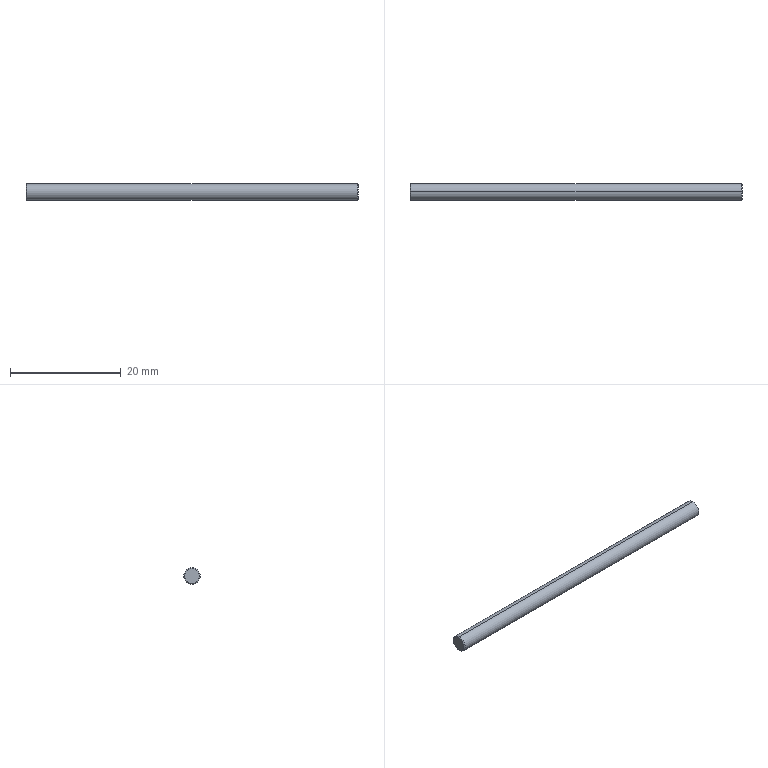Part | SolidWorks | features Chamfer 1, Extrusion 1 | 1 solid | 8 faces | box 60 x 3 x 3 mm | volume 423.91 mm3 | cone 4 | cylinder 2 | plane 2 | commonest cylinder face diameters 3 x2
STEP:
#1=CARTESIAN_POINT('',(30.,0.,-1.35));
#2=VERTEX_POINT('',#1);
#3=CARTESIAN_POINT('',(30.,0.,1.35));
#4=VERTEX_POINT('',#3);
#5=CARTESIAN_POINT('',(30.,0.,0.));
#6=DIRECTION('',(1.,0.,0.));
#7=DIRECTION('',(0.,0.,-1.));
#8=AXIS2_PLACEMENT_3D('',#5,#6,#7);
#9=CIRCLE('',#8,1.35);
#10=EDGE_CURVE('',#2,#4,#9,.T.);
#11=ORIENTED_EDGE('',*,*,#10,.F.);
#12=CARTESIAN_POINT('',(29.85,0.,-1.5));
#13=VERTEX_POINT('',#12);
#14=CARTESIAN_POINT('',(30.,0.,-1.35));
#15=DIRECTION('',(-0.7071,0.,-0.7071));
#16=VECTOR('',#15,1000.);
#17=LINE('',#14,#16);
#18=EDGE_CURVE('',#2,#13,#17,.T.);
#19=ORIENTED_EDGE('',*,*,#18,.T.);
#20=CARTESIAN_POINT('',(29.85,0.,1.5));
#21=VERTEX_POINT('',#20);
#22=CARTESIAN_POINT('',(29.85,0.,0.));
#23=DIRECTION('',(-1.,0.,0.));
#24=DIRECTION('',(0.,0.,-1.));
#25=AXIS2_PLACEMENT_3D('',#22,#23,#24);
#26=CIRCLE('',#25,1.5);
#27=EDGE_CURVE('',#21,#13,#26,.T.);
#28=ORIENTED_EDGE('',*,*,#27,.F.);
#29=CARTESIAN_POINT('',(30.,0.,1.35));
#30=DIRECTION('',(-0.7071,0.,0.7071));
#31=VECTOR('',#30,1000.);
#32=LINE('',#29,#31);
#33=EDGE_CURVE('',#4,#21,#32,.T.);
#34=ORIENTED_EDGE('',*,*,#33,.F.);
#35=EDGE_LOOP('',(#11,#19,#28,#34));
#36=FACE_OUTER_BOUND('',#35,.T.);
#37=CARTESIAN_POINT('',(30.,0.,0.));
#38=DIRECTION('',(-1.,0.,0.));
#39=DIRECTION('',(0.,0.,1.));
#40=AXIS2_PLACEMENT_3D('',#37,#38,#39);
#41=CONICAL_SURFACE('',#40,1.35,0.7854);
#42=ADVANCED_FACE('',(#36),#41,.T.);
#43=CARTESIAN_POINT('',(-30.,0.,1.35));
#44=VERTEX_POINT('',#43);
#45=CARTESIAN_POINT('',(-30.,0.,-1.35));
#46=VERTEX_POINT('',#45);
#47=CARTESIAN_POINT('',(-30.,0.,0.));
#48=DIRECTION('',(-1.,0.,0.));
#49=DIRECTION('',(0.,0.,-1.));
#50=AXIS2_PLACEMENT_3D('',#47,#48,#49);
#51=CIRCLE('',#50,1.35);
#52=EDGE_CURVE('',#44,#46,#51,.T.);
#53=ORIENTED_EDGE('',*,*,#52,.F.);
#54=CARTESIAN_POINT('',(-29.85,0.,1.5));
#55=VERTEX_POINT('',#54);
#56=CARTESIAN_POINT('',(-29.85,0.,1.5));
#57=DIRECTION('',(0.7071,0.,0.7071));
#58=VECTOR('',#57,1000.);
#59=LINE('',#56,#58);
#60=EDGE_CURVE('',#44,#55,#59,.T.);
#61=ORIENTED_EDGE('',*,*,#60,.T.);
#62=CARTESIAN_POINT('',(-29.85,0.,-1.5));
#63=VERTEX_POINT('',#62);
#64=CARTESIAN_POINT('',(-29.85,0.,0.));
#65=DIRECTION('',(1.,0.,0.));
#66=DIRECTION('',(0.,0.,-1.));
#67=AXIS2_PLACEMENT_3D('',#64,#65,#66);
#68=CIRCLE('',#67,1.5);
#69=EDGE_CURVE('',#63,#55,#68,.T.);
#70=ORIENTED_EDGE('',*,*,#69,.F.);
#71=CARTESIAN_POINT('',(-29.85,0.,-1.5));
#72=DIRECTION('',(0.7071,0.,-0.7071));
#73=VECTOR('',#72,1000.);
#74=LINE('',#71,#73);
#75=EDGE_CURVE('',#46,#63,#74,.T.);
#76=ORIENTED_EDGE('',*,*,#75,.F.);
#77=EDGE_LOOP('',(#53,#61,#70,#76));
#78=FACE_OUTER_BOUND('',#77,.T.);
#79=CARTESIAN_POINT('',(-29.85,0.,0.));
#80=DIRECTION('',(1.,0.,0.));
#81=DIRECTION('',(0.,0.,-1.));
#82=AXIS2_PLACEMENT_3D('',#79,#80,#81);
#83=CONICAL_SURFACE('',#82,1.5,0.7854);
#84=ADVANCED_FACE('',(#78),#83,.T.);
#85=ORIENTED_EDGE('',*,*,#27,.T.);
#86=CARTESIAN_POINT('',(30.,0.,-1.5));
#87=DIRECTION('',(-1.,0.,0.));
#88=VECTOR('',#87,1000.);
#89=LINE('',#86,#88);
#90=EDGE_CURVE('',#13,#63,#89,.T.);
#91=ORIENTED_EDGE('',*,*,#90,.T.);
#92=ORIENTED_EDGE('',*,*,#69,.T.);
#93=CARTESIAN_POINT('',(30.,0.,1.5));
#94=DIRECTION('',(-1.,0.,0.));
#95=VECTOR('',#94,1000.);
#96=LINE('',#93,#95);
#97=EDGE_CURVE('',#21,#55,#96,.T.);
#98=ORIENTED_EDGE('',*,*,#97,.F.);
#99=EDGE_LOOP('',(#85,#91,#92,#98));
#100=FACE_OUTER_BOUND('',#99,.T.);
#101=CARTESIAN_POINT('',(30.,0.,0.));
#102=DIRECTION('',(-1.,0.,0.));
#103=DIRECTION('',(0.,0.,1.));
#104=AXIS2_PLACEMENT_3D('',#101,#102,#103);
#105=CYLINDRICAL_SURFACE('',#104,1.5);
#106=ADVANCED_FACE('',(#100),#105,.T.);
#107=ORIENTED_EDGE('',*,*,#90,.F.);
#108=CARTESIAN_POINT('',(29.85,0.,0.));
#109=DIRECTION('',(-1.,0.,0.));
#110=DIRECTION('',(0.,0.,-1.));
#111=AXIS2_PLACEMENT_3D('',#108,#109,#110);
#112=CIRCLE('',#111,1.5);
#113=EDGE_CURVE('',#13,#21,#112,.T.);
#114=ORIENTED_EDGE('',*,*,#113,.T.);
#115=ORIENTED_EDGE('',*,*,#97,.T.);
#116=CARTESIAN_POINT('',(-29.85,0.,0.));
#117=DIRECTION('',(1.,0.,0.));
#118=DIRECTION('',(0.,0.,-1.));
#119=AXIS2_PLACEMENT_3D('',#116,#117,#118);
#120=CIRCLE('',#119,1.5);
#121=EDGE_CURVE('',#55,#63,#120,.T.);
#122=ORIENTED_EDGE('',*,*,#121,.T.);
#123=EDGE_LOOP('',(#107,#114,#115,#122));
#124=FACE_OUTER_BOUND('',#123,.T.);
#125=CARTESIAN_POINT('',(30.,0.,0.));
#126=DIRECTION('',(-1.,0.,0.));
#127=DIRECTION('',(0.,0.,1.));
#128=AXIS2_PLACEMENT_3D('',#125,#126,#127);
#129=CYLINDRICAL_SURFACE('',#128,1.5);
#130=ADVANCED_FACE('',(#124),#129,.T.);
#131=CARTESIAN_POINT('',(30.,0.,0.));
#132=DIRECTION('',(1.,0.,0.));
#133=DIRECTION('',(0.,0.,-1.));
#134=AXIS2_PLACEMENT_3D('',#131,#132,#133);
#135=CIRCLE('',#134,1.35);
#136=EDGE_CURVE('',#4,#2,#135,.T.);
#137=ORIENTED_EDGE('',*,*,#136,.T.);
#138=ORIENTED_EDGE('',*,*,#10,.T.);
#139=EDGE_LOOP('',(#137,#138));
#140=FACE_OUTER_BOUND('',#139,.T.);
#141=CARTESIAN_POINT('',(30.,0.,0.));
#142=DIRECTION('',(1.,0.,0.));
#143=DIRECTION('',(0.,0.,-1.));
#144=AXIS2_PLACEMENT_3D('',#141,#142,#143);
#145=PLANE('',#144);
#146=ADVANCED_FACE('',(#140),#145,.T.);
#147=CARTESIAN_POINT('',(-30.,0.,0.));
#148=DIRECTION('',(-1.,0.,0.));
#149=DIRECTION('',(0.,0.,-1.));
#150=AXIS2_PLACEMENT_3D('',#147,#148,#149);
#151=CIRCLE('',#150,1.35);
#152=EDGE_CURVE('',#46,#44,#151,.T.);
#153=ORIENTED_EDGE('',*,*,#152,.T.);
#154=ORIENTED_EDGE('',*,*,#52,.T.);
#155=EDGE_LOOP('',(#153,#154));
#156=FACE_OUTER_BOUND('',#155,.T.);
#157=CARTESIAN_POINT('',(-30.,0.,0.));
#158=DIRECTION('',(1.,0.,0.));
#159=DIRECTION('',(0.,0.,-1.));
#160=AXIS2_PLACEMENT_3D('',#157,#158,#159);
#161=PLANE('',#160);
#162=ADVANCED_FACE('',(#156),#161,.F.);
#163=ORIENTED_EDGE('',*,*,#60,.F.);
#164=ORIENTED_EDGE('',*,*,#152,.F.);
#165=ORIENTED_EDGE('',*,*,#75,.T.);
#166=ORIENTED_EDGE('',*,*,#121,.F.);
#167=EDGE_LOOP('',(#163,#164,#165,#166));
#168=FACE_OUTER_BOUND('',#167,.T.);
#169=CARTESIAN_POINT('',(-29.85,0.,0.));
#170=DIRECTION('',(1.,0.,0.));
#171=DIRECTION('',(0.,0.,-1.));
#172=AXIS2_PLACEMENT_3D('',#169,#170,#171);
#173=CONICAL_SURFACE('',#172,1.5,0.7854);
#174=ADVANCED_FACE('',(#168),#173,.T.);
#175=ORIENTED_EDGE('',*,*,#18,.F.);
#176=ORIENTED_EDGE('',*,*,#136,.F.);
#177=ORIENTED_EDGE('',*,*,#33,.T.);
#178=ORIENTED_EDGE('',*,*,#113,.F.);
#179=EDGE_LOOP('',(#175,#176,#177,#178));
#180=FACE_OUTER_BOUND('',#179,.T.);
#181=CARTESIAN_POINT('',(30.,0.,0.));
#182=DIRECTION('',(-1.,0.,0.));
#183=DIRECTION('',(0.,0.,1.));
#184=AXIS2_PLACEMENT_3D('',#181,#182,#183);
#185=CONICAL_SURFACE('',#184,1.35,0.7854);
#186=ADVANCED_FACE('',(#180),#185,.T.);
#187=CLOSED_SHELL('',(#42,#84,#106,#130,#146,#162,#174,#186));
#188=MANIFOLD_SOLID_BREP('',#187);
#189=CARTESIAN_POINT('',(0.,0.,0.));
#190=DIRECTION('',(0.,0.,1.));
#191=DIRECTION('',(1.,0.,0.));
#192=AXIS2_PLACEMENT_3D('',#189,#190,#191);
#193=(LENGTH_UNIT()NAMED_UNIT(*)SI_UNIT(.MILLI.,.METRE.));
#194=UNCERTAINTY_MEASURE_WITH_UNIT(LENGTH_MEASURE(0.00001),#193,'','');
#195=(NAMED_UNIT(*)PLANE_ANGLE_UNIT()SI_UNIT($,.RADIAN.));
#196=(NAMED_UNIT(*)SI_UNIT($,.STERADIAN.)SOLID_ANGLE_UNIT());
#197=(GEOMETRIC_REPRESENTATION_CONTEXT(3)GLOBAL_UNCERTAINTY_ASSIGNED_CONTEXT((#194))GLOBAL_UNIT_ASSIGNED_CONTEXT((#193,#195,#196))REPRESENTATION_CONTEXT('',''));
#198=ADVANCED_BREP_SHAPE_REPRESENTATION('',(#188,#192),#197);